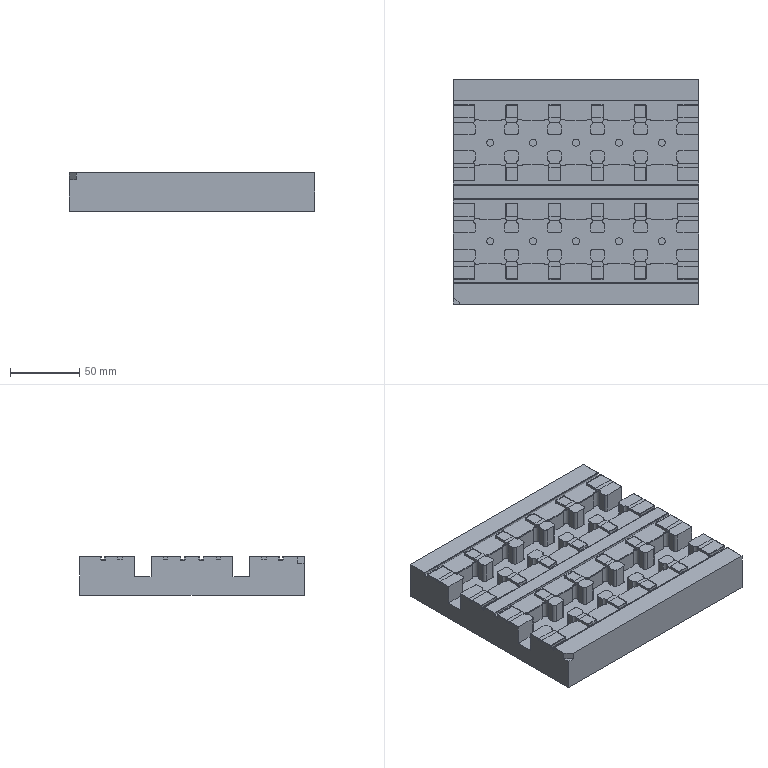NC program | NX | posted by the shop | part box 177 x 162 x 28 mm
Lines 249523 to 252035 of 254847:
N6 T04 M06
(D3  D=3. R=0. H=04 ce=0.05 di=0.02)
(D.N=04 MAX_Z=43. MIN_Z=25.32 Time=23.67M)
T17
G00 G90 G54 X94. Y64.15 M03 S5000
G43 H04 Z43.
M08
Z27.94
G01 X88.5 F1500.
X-88.5
X-94.
G00 Z27.88
G01 X-88.5
X88.5
X94.
G00 Z27.82
G01 X88.5
X-88.5
X-94.
G00 Z27.76
G01 X-88.5
X88.5
X94.
G00 Z27.7
G01 X88.5
X-88.5
X-94.
G00 Z27.64
G01 X-88.5
X88.5
X94.
G00 Z27.58
G01 X88.5
X-88.5
X-94.
G00 Z27.52
G01 X-88.5
X88.5
X94.
G00 Z27.46
G01 X88.5
X-88.5
X-94.
G00 Z27.4
G01 X-88.5
X88.5
X94.
G00 Z27.34
G01 X88.5
X-88.5
X-94.
G00 Z27.28
G01 X-88.5
X88.5
X94.
G00 Z27.22
G01 X88.5
X-88.5
X-94.
G00 Z27.16
G01 X-88.5
X88.5
X94.
G00 Z27.1
G01 X88.5
X-88.5
X-94.
G00 Z27.04
G01 X-88.5
X88.5
X94.
G00 Z26.98
G01 X88.5
X-88.5
X-94.
G00 Z26.92
G01 X-88.5
X88.5
X94.
G00 Z26.86
G01 X88.5
X-88.5
X-94.
G00 Z26.8
G01 X-88.5
X88.5
X94.
G00 Z26.74
G01 X88.5
X-88.5
X-94.
G00 Z26.68
G01 X-88.5
X88.5
X94.
G00 Z26.62
G01 X88.5
X-88.5
X-94.
G00 Z26.56
G01 X-88.5
X88.5
X94.
G00 Z26.5
G01 X88.5
X-88.5
X-94.
G00 Z26.44
G01 X-88.5
X88.5
X94.
G00 Z26.38
G01 X88.5
X-88.5
X-94.
G00 Z26.32
G01 X-88.5
X88.5
X94.
G00 Z26.26
G01 X88.5
X-88.5
X-94.
G00 Z26.2
G01 X-88.5
X88.5
X94.
G00 Z26.14
G01 X88.5
X-88.5
X-94.
G00 Z26.08
G01 X-88.5
X88.5
X94.
G00 Z26.02
G01 X88.5
X-88.5
X-94.
G00 Z25.96
G01 X-88.5
X88.5
X94.
G00 Z25.9
G01 X88.5
X-88.5
X-94.
G00 Z25.84
G01 X-88.5
X88.5
X94.
G00 Z25.78
G01 X88.5
X-88.5
X-94.
G00 Z25.72
G01 X-88.5
X88.5
X94.
G00 Z25.66
G01 X88.5
X-88.5
X-94.
G00 Z25.6
G01 X-88.5
X88.5
X94.
G00 Z25.54
G01 X88.5
X-88.5
X-94.
G00 Z25.48
G01 X-88.5
X88.5
X94.
G00 Z25.42
G01 X88.5
X-88.5
X-94.
G00 Z25.36
G01 X-88.5
X88.5
X94.
G00 Z25.32
G01 X88.5
X-88.5
X-94.
G00 Z43.
Y7.05
Z27.94
G01 X-88.5
X88.5
X94.
G00 Z27.88
G01 X88.5
X-88.5
X-94.
G00 Z27.82
G01 X-88.5
X88.5
X94.
G00 Z27.76
G01 X88.5
X-88.5
X-94.
G00 Z27.7
G01 X-88.5
X88.5
X94.
G00 Z27.64
G01 X88.5
X-88.5
X-94.
G00 Z27.58
G01 X-88.5
X88.5
X94.
G00 Z27.52
G01 X88.5
X-88.5
X-94.
G00 Z27.46
G01 X-88.5
X88.5
X94.
G00 Z27.4
G01 X88.5
X-88.5
X-94.
G00 Z27.34
G01 X-88.5
X88.5
X94.
G00 Z27.28
G01 X88.5
X-88.5
X-94.
G00 Z27.22
G01 X-88.5
X88.5
X94.
G00 Z27.16
G01 X88.5
X-88.5
X-94.
G00 Z27.1
G01 X-88.5
X88.5
X94.
G00 Z27.04
G01 X88.5
X-88.5
X-94.
G00 Z26.98
G01 X-88.5
X88.5
X94.
G00 Z26.92
G01 X88.5
X-88.5
X-94.
G00 Z26.86
G01 X-88.5
X88.5
X94.
G00 Z26.8
G01 X88.5
X-88.5
X-94.
G00 Z26.74
G01 X-88.5
X88.5
X94.
G00 Z26.68
G01 X88.5
X-88.5
X-94.
G00 Z26.62
G01 X-88.5
X88.5
X94.
G00 Z26.56
G01 X88.5
X-88.5
X-94.
G00 Z26.5
G01 X-88.5
X88.5
X94.
G00 Z26.44
G01 X88.5
X-88.5
X-94.
G00 Z26.38
G01 X-88.5
X88.5
X94.
G00 Z26.32
G01 X88.5
X-88.5
X-94.
G00 Z26.26
G01 X-88.5
X88.5
X94.
G00 Z26.2
G01 X88.5
X-88.5
X-94.
G00 Z26.14
G01 X-88.5
X88.5
X94.
G00 Z26.08
G01 X88.5
X-88.5
X-94.
G00 Z26.02
G01 X-88.5
X88.5
X94.
G00 Z25.96
G01 X88.5
X-88.5
X-94.
G00 Z25.9
G01 X-88.5
X88.5
X94.
G00 Z25.84
G01 X88.5
X-88.5
X-94.
G00 Z25.78
G01 X-88.5
X88.5
X94.
G00 Z25.72
G01 X88.5
X-88.5
X-94.
G00 Z25.66
G01 X-88.5
X88.5
X94.
G00 Z25.6
G01 X88.5
X-88.5
X-94.
G00 Z25.54
G01 X-88.5
X88.5
X94.
G00 Z25.48
G01 X88.5
X-88.5
X-94.
G00 Z25.42
G01 X-88.5
X88.5
X94.
G00 Z25.36
G01 X88.5
X-88.5
X-94.
G00 Z25.32
G01 X-88.5
X88.5
X94.
G00 Z43.
Y-7.05
Z27.94
G01 X88.5
X-88.5
X-94.
G00 Z27.88
G01 X-88.5
X88.5
X94.
G00 Z27.82
G01 X88.5
X-88.5
X-94.
G00 Z27.76
G01 X-88.5
X88.5
X94.
G00 Z27.7
G01 X88.5
X-88.5
X-94.
G00 Z27.64
G01 X-88.5
X88.5
X94.
G00 Z27.58
G01 X88.5
X-88.5
X-94.
G00 Z27.52
G01 X-88.5
X88.5
X94.
G00 Z27.46
G01 X88.5
X-88.5
X-94.
G00 Z27.4
G01 X-88.5
X88.5
X94.
G00 Z27.34
G01 X88.5
X-88.5
X-94.
G00 Z27.28
G01 X-88.5
X88.5
X94.
G00 Z27.22
G01 X88.5
X-88.5
X-94.
G00 Z27.16
G01 X-88.5
X88.5
X94.
G00 Z27.1
G01 X88.5
X-88.5
X-94.
G00 Z27.04
G01 X-88.5
X88.5
X94.
G00 Z26.98
G01 X88.5
X-88.5
X-94.
G00 Z26.92
G01 X-88.5
X88.5
X94.
G00 Z26.86
G01 X88.5
X-88.5
X-94.
G00 Z26.8
G01 X-88.5
X88.5
X94.
G00 Z26.74
G01 X88.5
X-88.5
X-94.
G00 Z26.68
G01 X-88.5
X88.5
X94.
G00 Z26.62
G01 X88.5
X-88.5
X-94.
G00 Z26.56
G01 X-88.5
X88.5
X94.
G00 Z26.5
G01 X88.5
X-88.5
X-94.
G00 Z26.44
G01 X-88.5
X88.5
X94.
G00 Z26.38
G01 X88.5
X-88.5
X-94.
G00 Z26.32
G01 X-88.5
X88.5
X94.
G00 Z26.26
G01 X88.5
X-88.5
X-94.
G00 Z26.2
G01 X-88.5
X88.5
X94.
G00 Z26.14
G01 X88.5
X-88.5
X-94.
G00 Z26.08
G01 X-88.5
X88.5
X94.
G00 Z26.02
G01 X88.5
X-88.5
X-94.
G00 Z25.96
G01 X-88.5
X88.5
X94.
G00 Z25.9
G01 X88.5
X-88.5
X-94.
G00 Z25.84
G01 X-88.5
X88.5
X94.
G00 Z25.78
G01 X88.5
X-88.5
X-94.
G00 Z25.72
G01 X-88.5
X88.5
X94.
G00 Z25.66
G01 X88.5
X-88.5
X-94.
G00 Z25.6
G01 X-88.5
X88.5
X94.
G00 Z25.54
G01 X88.5
X-88.5
X-94.
G00 Z25.48
G01 X-88.5
X88.5
X94.
G00 Z25.42
G01 X88.5
X-88.5
X-94.
G00 Z25.36
G01 X-88.5
X88.5
X94.
G00 Z25.32
G01 X88.5
X-88.5
X-94.
G00 Z43.
Y-64.15
Z27.94
G01 X-88.5
X88.5
X94.
G00 Z27.88
G01 X88.5
X-88.5
X-94.
G00 Z27.82
G01 X-88.5
X88.5
X94.
G00 Z27.76
G01 X88.5
X-88.5
X-94.
G00 Z27.7
G01 X-88.5
X88.5
X94.
G00 Z27.64
G01 X88.5
X-88.5
X-94.
G00 Z27.58
G01 X-88.5
X88.5
X94.
G00 Z27.52
G01 X88.5
X-88.5
X-94.
G00 Z27.46
G01 X-88.5
X88.5
X94.
G00 Z27.4
G01 X88.5
X-88.5
X-94.
G00 Z27.34
G01 X-88.5
X88.5
X94.
G00 Z27.28
G01 X88.5
X-88.5
X-94.
G00 Z27.22
G01 X-88.5
X88.5
X94.
G00 Z27.16
G01 X88.5
X-88.5
X-94.
G00 Z27.1
G01 X-88.5
X88.5
X94.
G00 Z27.04
G01 X88.5
X-88.5
X-94.
G00 Z26.98
G01 X-88.5
X88.5
X94.
G00 Z26.92
G01 X88.5
X-88.5
X-94.
G00 Z26.86
G01 X-88.5
X88.5
X94.
G00 Z26.8
G01 X88.5
X-88.5
X-94.
G00 Z26.74
G01 X-88.5
X88.5
X94.
G00 Z26.68
G01 X88.5
X-88.5
X-94.
G00 Z26.62
G01 X-88.5
X88.5
X94.
G00 Z26.56
G01 X88.5
X-88.5
X-94.
G00 Z26.5
G01 X-88.5
X88.5
X94.
G00 Z26.44
G01 X88.5
X-88.5
X-94.
G00 Z26.38
G01 X-88.5
X88.5
X94.
G00 Z26.32
G01 X88.5
X-88.5
X-94.
G00 Z26.26
G01 X-88.5
X88.5
X94.
G00 Z26.2
G01 X88.5
X-88.5
X-94.
G00 Z26.14
G01 X-88.5
X88.5
X94.
G00 Z26.08
G01 X88.5
X-88.5
X-94.
G00 Z26.02
G01 X-88.5
X88.5
X94.
G00 Z25.96
G01 X88.5
X-88.5
X-94.
G00 Z25.9
G01 X-88.5
X88.5
X94.
G00 Z25.84
G01 X88.5
X-88.5
X-94.
G00 Z25.78
G01 X-88.5
X88.5
X94.
G00 Z25.72
G01 X88.5
X-88.5
X-94.
G00 Z25.66
G01 X-88.5
X88.5
X94.
G00 Z25.6
G01 X88.5
X-88.5
X-94.
G00 Z25.54
G01 X-88.5
X88.5
X94.
G00 Z25.48
G01 X88.5
X-88.5
X-94.
G00 Z25.42
G01 X-88.5
X88.5
X94.
G00 Z25.36
G01 X88.5
X-88.5
X-94.
G00 Z25.32
G01 X-88.5
X88.5
X94.
G00 Z43.
G00 G90 X71.136 Y50.333 M03 S5000
Z40.
Z26.35
G01 Z25.35 F1000.
G41 D04
X71.276 Y50.475
G03 X71.45 Y50.897 I-.426 J.422
G01 Y64.15
X52.55
Y50.897
G03 X52.724 Y50.475 I.6 J0.0
G01 G40 X52.864 Y50.333
Z26.35
G00 Z40.
X40.136
Z26.35
G01 Z25.35
G41 D04
X40.276 Y50.475
G03 X40.45 Y50.897 I-.426 J.422
G01 Y64.15
X21.55
Y50.897
G03 X21.724 Y50.475 I.6 J0.0
G01 G40 X21.864 Y50.333
Z26.35
G00 Z40.
X9.136
Z26.35
G01 Z25.35
G41 D04
X9.276 Y50.475
G03 X9.45 Y50.897 I-.426 J.422
G01 Y64.15
X-9.45
Y50.897
G03 X-9.276 Y50.475 I.6 J0.0
G01 G40 X-9.136 Y50.333
Z26.35
G00 Z40.
X-21.864
Z26.35
G01 Z25.35
G41 D04
X-21.724 Y50.475
G03 X-21.55 Y50.897 I-.426 J.422
G01 Y64.15
X-40.45
Y50.897
G03 X-40.276 Y50.475 I.6 J0.0
G01 G40 X-40.136 Y50.333
Z26.35
G00 Z40.
X-52.864
Z26.35
G01 Z25.35
G41 D04
X-52.724 Y50.475
G03 X-52.55 Y50.897 I-.426 J.422
G01 Y64.15
X-71.45
Y50.897
G03 X-71.276 Y50.475 I.6 J0.0
G01 G40 X-71.136 Y50.333
Z26.35
G00 Z40.
X52.864 Y20.867
Z26.35
G01 Z25.35
G41 D04
X52.724 Y20.725
G03 X52.55 Y20.303 I.426 J-.422
G01 Y7.05
X71.45
Y20.303
G03 X71.276 Y20.725 I-.6 J0.0
G01 G40 X71.136 Y20.867
Z26.35
G00 Z40.
X21.864
Z26.35
G01 Z25.35
G41 D04
X21.724 Y20.725
G03 X21.55 Y20.303 I.426 J-.422
G01 Y7.05
X40.45
Y20.303
G03 X40.276 Y20.725 I-.6 J0.0
G01 G40 X40.136 Y20.867
Z26.35
G00 Z40.
X-9.136
Z26.35
G01 Z25.35
G41 D04
X-9.276 Y20.725
G03 X-9.45 Y20.303 I.426 J-.422
G01 Y7.05
X9.45
Y20.303
G03 X9.276 Y20.725 I-.6 J0.0
G01 G40 X9.136 Y20.867
Z26.35
G00 Z40.
X-40.136
Z26.35
G01 Z25.35
G41 D04
X-40.276 Y20.725
G03 X-40.45 Y20.303 I.426 J-.422
G01 Y7.05
X-21.55
Y20.303
G03 X-21.724 Y20.725 I-.6 J0.0
G01 G40 X-21.864 Y20.867
Z26.35
G00 Z40.
X-71.136
Z26.35
G01 Z25.35
G41 D04
X-71.276 Y20.725
G03 X-71.45 Y20.303 I.426 J-.422
G01 Y7.05
X-52.55
Y20.303
G03 X-52.724 Y20.725 I-.6 J0.0
G01 G40 X-52.864 Y20.867
Z26.35
G00 Z40.
Y-20.867
Z26.35
G01 Z25.35
G41 D04
X-52.724 Y-20.725
G03 X-52.55 Y-20.303 I-.426 J.422
G01 Y-7.05
X-71.45
Y-20.303
G03 X-71.276 Y-20.725 I.6 J0.0
G01 G40 X-71.136 Y-20.867
Z26.35
G00 Z40.
X-21.864
Z26.35
G01 Z25.35
G41 D04
X-21.724 Y-20.725
G03 X-21.55 Y-20.303 I-.426 J.422
G01 Y-7.05
X-40.45
Y-20.303
G03 X-40.276 Y-20.725 I.6 J0.0
G01 G40 X-40.136 Y-20.867
Z26.35
G00 Z40.
X9.136
Z26.35
G01 Z25.35
G41 D04
X9.276 Y-20.725
G03 X9.45 Y-20.303 I-.426 J.422
G01 Y-7.05
X-9.45
Y-20.303
G03 X-9.276 Y-20.725 I.6 J0.0
G01 G40 X-9.136 Y-20.867
Z26.35
G00 Z40.
X40.136
Z26.35
G01 Z25.35
G41 D04
X40.276 Y-20.725
G03 X40.45 Y-20.303 I-.426 J.422
G01 Y-7.05
X21.55
Y-20.303
G03 X21.724 Y-20.725 I.6 J0.0
G01 G40 X21.864 Y-20.867
Z26.35
G00 Z40.
X71.136
Z26.35
G01 Z25.35
G41 D04
X71.276 Y-20.725
G03 X71.45 Y-20.303 I-.426 J.422
G01 Y-7.05
X52.55
Y-20.303
G03 X52.724 Y-20.725 I.6 J0.0
G01 G40 X52.864 Y-20.867
Z26.35
G00 Z40.
Y-50.333
Z26.35
G01 Z25.35
G41 D04
X52.724 Y-50.475
G03 X52.55 Y-50.897 I.426 J-.422
G01 Y-64.15
X71.45
Y-50.897
G03 X71.276 Y-50.475 I-.6 J0.0
G01 G40 X71.136 Y-50.333
Z26.35
G00 Z40.
X21.864
Z26.35
G01 Z25.35
G41 D04
X21.724 Y-50.475
G03 X21.55 Y-50.897 I.426 J-.422
G01 Y-64.15
X40.45
Y-50.897
G03 X40.276 Y-50.475 I-.6 J0.0
G01 G40 X40.136 Y-50.333
Z26.35
G00 Z40.
X-9.136
Z26.35
G01 Z25.35
G41 D04
X-9.276 Y-50.475
G03 X-9.45 Y-50.897 I.426 J-.422
G01 Y-64.15
X9.45
Y-50.897
G03 X9.276 Y-50.475 I-.6 J0.0
G01 G40 X9.136 Y-50.333
Z26.35
G00 Z40.
X-40.136
Z26.35
G01 Z25.35
G41 D04
X-40.276 Y-50.475
G03 X-40.45 Y-50.897 I.426 J-.422
G01 Y-64.15
X-21.55
Y-50.897
G03 X-21.724 Y-50.475 I-.6 J0.0
G01 G40 X-21.864 Y-50.333
Z26.35
G00 Z40.
X-71.136
Z26.35
G01 Z25.35
G41 D04
X-71.276 Y-50.475
G03 X-71.45 Y-50.897 I.426 J-.422
G01 Y-64.15
X-52.55
Y-50.897
G03 X-52.724 Y-50.475 I-.6 J0.0
G01 G40 X-52.864 Y-50.333
Z26.35
G00 Z40.
G91 G28 Z0.0
M05
M09
G91 G28 Z0.0
M01
N7 T17 M06
(C6SpotDrill  D=6. R=0. H=17 ce=0.00 di=0.05)
(MAX_Z=43. MIN_Z=12.7 Time=0.33M)
T03
G00 G90 G54 X-62. Y-35.6 M03 S1500
G43 H17 Z43.
M08
G98 G81 X-62. Y-35.6 Z12.7 R14.5 F60.
X-31.
X0.0
X31.
X62.
Y35.6
X31.
X0.0
X-31.
X-62.
G80
G00 Z43.
G91 G28 Z0.0
M05
M09
G91 G28 Z0.0
M01
N8 T03 M06
(ZT5.1 D=5.1 DR_a=118 H=03)
(MAX_Z=43. MIN_Z=1.35 Time=1.12M)
T11
G00 G90 G54 X-62. Y-35.6 M03 S1200
G43 H03 Z43.
M08
G98 G83 X-62. Y-35.6 Z1.35 R14.5 F120. Q1.5
X-31.
X0.0
X31.
X62.
G98 G83 X62. Y35.6 Z1.6 R14.5 Q1.5
X31.
X0.0
X-31.
X-62.
G80
G00 Z43.
G91 G28 Z0.0
M05
M09
G91 G28 Z0.0
M01
N9 T11 M06
(D10-J  D=10. R=0. H=11 ce=0.00 di=0.00)
(MAX_Z=43. MIN_Z=28. Time=6.55M)
T14
G00 G90 G54 X98.5 Y-81.086 M03 S3000
G43 H11 Z43.
M08
Z30.
G01 Z28. F1000.
X93.5
X-93.5
Y-76.171
X93.5
Y-71.257
X-93.5
Y-66.343
X93.5
Y-61.429
X-93.5
Y-56.514
X93.5
Y-51.6
X-93.5
Y-46.686
X93.5
Y-41.771
X-93.5
Y-36.857
X93.5
Y-31.943
X-93.5
Y-27.029
X93.5
Y-22.114
X-93.5
Y-17.2
X93.5
Y-12.286
X-93.5
Y-7.371
X93.5
Y-2.457
X-93.5
Y2.457
X93.5
Y7.371
X-93.5
Y12.286
X93.5
Y17.2
X-93.5
Y22.114
X93.5
Y27.029
X-93.5
Y31.943
X93.5
Y36.857
X-93.5
Y41.771
X93.5
Y46.686
X-93.5
Y51.6
X93.5
Y56.514
X-93.5
Y61.429
X93.5
Y66.343
X-93.5
Y71.257
X93.5
Y76.171
X-93.5
Y81.086
X93.5
X98.5
Z30.
G00 Z43.
G91 G28 Z0.0
M05
M09
G91 G28 Z0.0
M01
N10 T14 M06
(D4-J  D=4. R=0. H=14 ce=0.30 di=0.00)
(MAX_Z=43. MIN_Z=13.5 Time=3.21M)
T13
G00 G90 G54 X-93.5 Y35.6 M03 S4000
G43 H14 Z43.
M08
Z14.
G01 Z13.5 F900.
X-88.9
Y39.3 F1000.
X-74.25
G03 X-69.95 Y43.6 I0.0 J4.3
G01 Y47.931
G03 X-70.334 Y49.204 I-2.3 J0.0
X-69.561 Y49.07 I.773 J2.166
G01 X-54.439
G03 X-53.666 Y49.204 I0.0 J2.3
X-54.05 Y47.931 I1.916 J-1.273
G01 Y43.6
G03 X-49.75 Y39.3 I4.3 J0.0
G01 X-43.25
G03 X-38.95 Y43.6 I0.0 J4.3
G01 Y47.931
G03 X-39.334 Y49.204 I-2.3 J0.0
X-38.561 Y49.07 I.773 J2.166
G01 X-23.439
G03 X-22.666 Y49.204 I0.0 J2.3
X-23.05 Y47.931 I1.916 J-1.273
G01 Y43.6
G03 X-18.75 Y39.3 I4.3 J0.0
G01 X-12.25
G03 X-7.95 Y43.6 I0.0 J4.3
G01 Y47.931
G03 X-8.334 Y49.204 I-2.3 J0.0
X-7.561 Y49.07 I.773 J2.166
G01 X7.561
G03 X8.334 Y49.204 I0.0 J2.3
X7.95 Y47.931 I1.916 J-1.273
G01 Y43.6
G03 X12.25 Y39.3 I4.3 J0.0
G01 X18.75
G03 X23.05 Y43.6 I0.0 J4.3
G01 Y47.931
G03 X22.666 Y49.204 I-2.3 J0.0
X23.439 Y49.07 I.773 J2.166
G01 X38.561
G03 X39.334 Y49.204 I0.0 J2.3
X38.95 Y47.931 I1.916 J-1.273
G01 Y43.6
G03 X43.25 Y39.3 I4.3 J0.0
G01 X49.75
G03 X54.05 Y43.6 I0.0 J4.3
G01 Y47.931
G03 X53.666 Y49.204 I-2.3 J0.0
X54.439 Y49.07 I.773 J2.166
G01 X69.561
G03 X70.334 Y49.204 I0.0 J2.3
X69.95 Y47.931 I1.916 J-1.273
G01 Y43.6
G03 X74.25 Y39.3 I4.3 J0.0
G01 X88.9
Y31.9
X74.25
G03 X69.95 Y27.6 I0.0 J-4.3
G01 Y23.269
G03 X70.334 Y21.996 I2.3 J0.0
X69.561 Y22.13 I-.773 J-2.166
G01 X54.439
G03 X53.666 Y21.996 I0.0 J-2.3
X54.05 Y23.269 I-1.916 J1.273
G01 Y27.6
G03 X49.75 Y31.9 I-4.3 J0.0
G01 X43.25
G03 X38.95 Y27.6 I0.0 J-4.3
G01 Y23.269
G03 X39.334 Y21.996 I2.3 J0.0
X38.561 Y22.13 I-.773 J-2.166
G01 X23.439
G03 X22.666 Y21.996 I0.0 J-2.3
X23.05 Y23.269 I-1.916 J1.273
G01 Y27.6
G03 X18.75 Y31.9 I-4.3 J0.0
G01 X12.25
G03 X7.95 Y27.6 I0.0 J-4.3
G01 Y23.269
G03 X8.334 Y21.996 I2.3 J0.0
X7.561 Y22.13 I-.773 J-2.166
G01 X-7.561
G03 X-8.334 Y21.996 I0.0 J-2.3
X-7.95 Y23.269 I-1.916 J1.273
G01 Y27.6
G03 X-12.25 Y31.9 I-4.3 J0.0
G01 X-18.75
G03 X-23.05 Y27.6 I0.0 J-4.3
G01 Y23.269
G03 X-22.666 Y21.996 I2.3 J0.0
X-23.439 Y22.13 I-.773 J-2.166
G01 X-38.561
G03 X-39.334 Y21.996 I0.0 J-2.3
X-38.95 Y23.269 I-1.916 J1.273
G01 Y27.6
G03 X-43.25 Y31.9 I-4.3 J0.0
G01 X-49.75
G03 X-54.05 Y27.6 I0.0 J-4.3
G01 Y23.269
G03 X-53.666 Y21.996 I2.3 J0.0
X-54.439 Y22.13 I-.773 J-2.166
G01 X-69.561
G03 X-70.334 Y21.996 I0.0 J-2.3
X-69.95 Y23.269 I-1.916 J1.273
G01 Y27.6
G03 X-74.25 Y31.9 I-4.3 J0.0
G01 X-88.9
Y35.6
X-86.8
Y37.2
X-74.25
G03 X-67.85 Y43.6 I0.0 J6.4
G01 Y46.97
X-56.15
Y43.6
G03 X-49.75 Y37.2 I6.4 J0.0
G01 X-43.25
G03 X-36.85 Y43.6 I0.0 J6.4
G01 Y46.97
X-25.15
Y43.6
G03 X-18.75 Y37.2 I6.4 J0.0
G01 X-12.25
G03 X-5.85 Y43.6 I0.0 J6.4
G01 Y46.97
X5.85
Y43.6
G03 X12.25 Y37.2 I6.4 J0.0
G01 X18.75
G03 X25.15 Y43.6 I0.0 J6.4
G01 Y46.97
X36.85
Y43.6
G03 X43.25 Y37.2 I6.4 J0.0
G01 X49.75
G03 X56.15 Y43.6 I0.0 J6.4
G01 Y46.97
X67.85
Y43.6
G03 X74.25 Y37.2 I6.4 J0.0
G01 X86.8
Y34.
X74.25
G03 X67.85 Y27.6 I0.0 J-6.4
G01 Y24.23
X56.15
Y27.6
G03 X52.91 Y33.165 I-6.4 J0.0
G01 X54.293 Y35.6
G03 X58.95 Y43.6 I-4.543 J8.
G01 Y44.17
X65.05
Y43.6
G03 X69.707 Y35.6 I9.2 J0.0
X65.05 Y27.6 I4.543 J-8.
G01 Y27.03
X58.95
Y27.6
G03 X54.293 Y35.6 I-9.2 J0.0
G01 X58.694
G03 X61.541 Y41.37 I-8.944 J8.
G01 X62.459
G03 X65.306 Y35.6 I11.791 J2.23
X62.459 Y29.83 I8.944 J-8.
G01 X61.541
G03 X58.694 Y35.6 I-11.791 J-2.23
G01 X60.995
G03 X62. Y37.246 I-11.245 J8.
X63.005 Y35.6 I12.25 J6.354
X62. Y33.954 I11.245 J-8.
X60.995 Y35.6 I-12.25 J-6.354
G01 X54.293
X52.91 Y33.165
G03 X49.75 Y34. I-3.16 J-5.565
G01 X43.25
G03 X36.85 Y27.6 I0.0 J-6.4
G01 Y24.23
X25.15
Y27.6
G03 X21.91 Y33.165 I-6.4 J0.0
G01 X23.293 Y35.6
G03 X27.95 Y43.6 I-4.543 J8.
G01 Y44.17
X34.05
Y43.6
G03 X38.707 Y35.6 I9.2 J0.0
X34.05 Y27.6 I4.543 J-8.
G01 Y27.03
X27.95
Y27.6
G03 X23.293 Y35.6 I-9.2 J0.0
G01 X27.694
G03 X30.541 Y41.37 I-8.944 J8.
G01 X31.459
G03 X34.306 Y35.6 I11.791 J2.23
X31.459 Y29.83 I8.944 J-8.
G01 X30.541
G03 X27.694 Y35.6 I-11.791 J-2.23
G01 X29.995
G03 X31. Y37.246 I-11.245 J8.
X32.005 Y35.6 I12.25 J6.354
X31. Y33.954 I11.245 J-8.
X29.995 Y35.6 I-12.25 J-6.354
G01 X23.293
X21.91 Y33.165
G03 X18.75 Y34. I-3.16 J-5.565
G01 X12.25
G03 X5.85 Y27.6 I0.0 J-6.4
G01 Y24.23
X-5.85
Y27.6
G03 X-9.09 Y33.165 I-6.4 J0.0
G01 X-7.707 Y35.6
G03 X-3.05 Y43.6 I-4.543 J8.
G01 Y44.17
X3.05
Y43.6
G03 X7.707 Y35.6 I9.2 J0.0
X3.05 Y27.6 I4.543 J-8.
G01 Y27.03
X-3.05
Y27.6
G03 X-7.707 Y35.6 I-9.2 J0.0
G01 X-3.306
G03 X-.459 Y41.37 I-8.944 J8.
G01 X.459
G03 X3.306 Y35.6 I11.791 J2.23
X.459 Y29.83 I8.944 J-8.
G01 X-.459
G03 X-3.306 Y35.6 I-11.791 J-2.23
G01 X-1.005
G03 X0.0 Y37.246 I-11.245 J8.
X1.005 Y35.6 I12.25 J6.354
X0.0 Y33.954 I11.245 J-8.
X-1.005 Y35.6 I-12.25 J-6.354
G01 X-7.707
X-9.09 Y33.165
G03 X-12.25 Y34. I-3.16 J-5.565
G01 X-18.75
G03 X-25.15 Y27.6 I0.0 J-6.4
G01 Y24.23
X-36.85
Y27.6
G03 X-40.09 Y33.165 I-6.4 J0.0
G01 X-38.707 Y35.6
G03 X-34.05 Y43.6 I-4.543 J8.
G01 Y44.17
X-27.95
Y43.6
G03 X-23.293 Y35.6 I9.2 J0.0
X-27.95 Y27.6 I4.543 J-8.
G01 Y27.03
X-34.05
Y27.6
G03 X-38.707 Y35.6 I-9.2 J0.0
G01 X-34.306
G03 X-31.459 Y41.37 I-8.944 J8.
G01 X-30.541
G03 X-27.694 Y35.6 I11.791 J2.23
X-30.541 Y29.83 I8.944 J-8.
G01 X-31.459
G03 X-34.306 Y35.6 I-11.791 J-2.23
G01 X-32.005
G03 X-31. Y37.246 I-11.245 J8.
X-29.995 Y35.6 I12.25 J6.354
X-31. Y33.954 I11.245 J-8.
X-32.005 Y35.6 I-12.25 J-6.354
G01 X-38.707
X-40.09 Y33.165
G03 X-43.25 Y34. I-3.16 J-5.565
G01 X-49.75
G03 X-56.15 Y27.6 I0.0 J-6.4
G01 Y24.23
X-67.85
Y27.6
G03 X-71.09 Y33.165 I-6.4 J0.0
G01 X-69.707 Y35.6
G03 X-65.05 Y43.6 I-4.543 J8.
G01 Y44.17
X-58.95
Y43.6
G03 X-54.293 Y35.6 I9.2 J0.0
X-58.95 Y27.6 I4.543 J-8.
G01 Y27.03
X-65.05
Y27.6
G03 X-69.707 Y35.6 I-9.2 J0.0
G01 X-65.306
G03 X-62.459 Y41.37 I-8.944 J8.
G01 X-61.541
G03 X-58.694 Y35.6 I11.791 J2.23
X-61.541 Y29.83 I8.944 J-8.
G01 X-62.459
G03 X-65.306 Y35.6 I-11.791 J-2.23
G01 X-63.005
G03 X-62. Y37.246 I-11.245 J8.
X-60.995 Y35.6 I12.25 J6.354
X-62. Y33.954 I11.245 J-8.
X-63.005 Y35.6 I-12.25 J-6.354
G01 X-69.707
X-71.09 Y33.165
G03 X-74.25 Y34. I-3.16 J-5.565
G01 X-86.8
Y35.6
Y36.1
X-93.5
Z14.
G00 Z43.
Y-35.6
Z14.
G01 Z13.5 F900.
X-88.9
Y-31.9 F1000.
X-74.25
G03 X-69.95 Y-27.6 I0.0 J4.3
G01 Y-23.269
G03 X-70.334 Y-21.996 I-2.3 J0.0
X-69.561 Y-22.13 I.773 J2.166
G01 X-54.439
G03 X-53.666 Y-21.996 I0.0 J2.3
X-54.05 Y-23.269 I1.916 J-1.273
G01 Y-27.6
G03 X-49.75 Y-31.9 I4.3 J0.0
G01 X-43.25
G03 X-38.95 Y-27.6 I0.0 J4.3
G01 Y-23.269
G03 X-39.334 Y-21.996 I-2.3 J0.0
X-38.561 Y-22.13 I.773 J2.166
G01 X-23.439
G03 X-22.666 Y-21.996 I0.0 J2.3
X-23.05 Y-23.269 I1.916 J-1.273
G01 Y-27.6
G03 X-18.75 Y-31.9 I4.3 J0.0
G01 X-12.25
G03 X-7.95 Y-27.6 I0.0 J4.3
G01 Y-23.269
G03 X-8.334 Y-21.996 I-2.3 J0.0
X-7.561 Y-22.13 I.773 J2.166
G01 X7.561
G03 X8.334 Y-21.996 I0.0 J2.3
X7.95 Y-23.269 I1.916 J-1.273
G01 Y-27.6
G03 X12.25 Y-31.9 I4.3 J0.0
G01 X18.75
G03 X23.05 Y-27.6 I0.0 J4.3
G01 Y-23.269
G03 X22.666 Y-21.996 I-2.3 J0.0
X23.439 Y-22.13 I.773 J2.166
G01 X38.561
G03 X39.334 Y-21.996 I0.0 J2.3
X38.95 Y-23.269 I1.916 J-1.273
G01 Y-27.6
G03 X43.25 Y-31.9 I4.3 J0.0
G01 X49.75
G03 X54.05 Y-27.6 I0.0 J4.3
G01 Y-23.269
G03 X53.666 Y-21.996 I-2.3 J0.0
X54.439 Y-22.13 I.773 J2.166
G01 X69.561
G03 X70.334 Y-21.996 I0.0 J2.3
X69.95 Y-23.269 I1.916 J-1.273
G01 Y-27.6
G03 X74.25 Y-31.9 I4.3 J0.0
G01 X88.9
Y-39.3
X74.25
G03 X69.95 Y-43.6 I0.0 J-4.3
G01 Y-47.931
G03 X70.334 Y-49.204 I2.3 J0.0
X69.561 Y-49.07 I-.773 J-2.166
G01 X54.439
G03 X53.666 Y-49.204 I0.0 J-2.3
X54.05 Y-47.931 I-1.916 J1.273
G01 Y-43.6
G03 X49.75 Y-39.3 I-4.3 J0.0
G01 X43.25
G03 X38.95 Y-43.6 I0.0 J-4.3
G01 Y-47.931
G03 X39.334 Y-49.204 I2.3 J0.0
X38.561 Y-49.07 I-.773 J-2.166
G01 X23.439
G03 X22.666 Y-49.204 I0.0 J-2.3
X23.05 Y-47.931 I-1.916 J1.273
G01 Y-43.6
G03 X18.75 Y-39.3 I-4.3 J0.0
G01 X12.25
G03 X7.95 Y-43.6 I0.0 J-4.3
G01 Y-47.931
G03 X8.334 Y-49.204 I2.3 J0.0
X7.561 Y-49.07 I-.773 J-2.166
G01 X-7.561
G03 X-8.334 Y-49.204 I0.0 J-2.3
X-7.95 Y-47.931 I-1.916 J1.273
G01 Y-43.6
G03 X-12.25 Y-39.3 I-4.3 J0.0
G01 X-18.75
G03 X-23.05 Y-43.6 I0.0 J-4.3
G01 Y-47.931
G03 X-22.666 Y-49.204 I2.3 J0.0
X-23.439 Y-49.07 I-.773 J-2.166
G01 X-38.561
G03 X-39.334 Y-49.204 I0.0 J-2.3
X-38.95 Y-47.931 I-1.916 J1.273
G01 Y-43.6
G03 X-43.25 Y-39.3 I-4.3 J0.0
G01 X-49.75
G03 X-54.05 Y-43.6 I0.0 J-4.3
G01 Y-47.931
G03 X-53.666 Y-49.204 I2.3 J0.0
X-54.439 Y-49.07 I-.773 J-2.166
G01 X-69.561
G03 X-70.334 Y-49.204 I0.0 J-2.3
X-69.95 Y-47.931 I-1.916 J1.273
G01 Y-43.6
G03 X-74.25 Y-39.3 I-4.3 J0.0
G01 X-88.9
Y-35.6
X-86.8
Y-34.
X-74.25
G03 X-67.85 Y-27.6 I0.0 J6.4
G01 Y-24.23
X-56.15
Y-27.6
G03 X-49.75 Y-34. I6.4 J0.0
G01 X-43.25
G03 X-36.85 Y-27.6 I0.0 J6.4
G01 Y-24.23
X-25.15
Y-27.6
G03 X-18.75 Y-34. I6.4 J0.0
G01 X-12.25
G03 X-5.85 Y-27.6 I0.0 J6.4
G01 Y-24.23
X5.85
Y-27.6
G03 X12.25 Y-34. I6.4 J0.0
G01 X18.75
G03 X25.15 Y-27.6 I0.0 J6.4
G01 Y-24.23
X36.85
Y-27.6
G03 X43.25 Y-34. I6.4 J0.0
G01 X49.75
G03 X56.15 Y-27.6 I0.0 J6.4
G01 Y-24.23
X67.85
Y-27.6
G03 X74.25 Y-34. I6.4 J0.0
G01 X86.8
Y-37.2
X74.25
G03 X67.85 Y-43.6 I0.0 J-6.4
G01 Y-46.97
X56.15
Y-43.6
G03 X52.91 Y-38.035 I-6.4 J0.0
G01 X54.293 Y-35.6
G03 X58.95 Y-27.6 I-4.543 J8.
G01 Y-27.03
X65.05
Y-27.6
G03 X69.707 Y-35.6 I9.2 J0.0
X65.05 Y-43.6 I4.543 J-8.
G01 Y-44.17
X58.95
Y-43.6
G03 X54.293 Y-35.6 I-9.2 J0.0
G01 X58.694
G03 X61.541 Y-29.83 I-8.944 J8.
G01 X62.459
G03 X65.306 Y-35.6 I11.791 J2.23
X62.459 Y-41.37 I8.944 J-8.
G01 X61.541
G03 X58.694 Y-35.6 I-11.791 J-2.23
G01 X60.995
G03 X62. Y-33.954 I-11.245 J8.
X63.005 Y-35.6 I12.25 J6.354
X62. Y-37.246 I11.245 J-8.
X60.995 Y-35.6 I-12.25 J-6.354
G01 X54.293
X52.91 Y-38.035
G03 X49.75 Y-37.2 I-3.16 J-5.565
G01 X43.25
G03 X36.85 Y-43.6 I0.0 J-6.4
G01 Y-46.97
X25.15
Y-43.6
G03 X21.91 Y-38.035 I-6.4 J0.0
G01 X23.293 Y-35.6
G03 X27.95 Y-27.6 I-4.543 J8.
G01 Y-27.03
X34.05
Y-27.6
G03 X38.707 Y-35.6 I9.2 J0.0
X34.05 Y-43.6 I4.543 J-8.
G01 Y-44.17
X27.95
Y-43.6
G03 X23.293 Y-35.6 I-9.2 J0.0
G01 X27.694
G03 X30.541 Y-29.83 I-8.944 J8.
G01 X31.459
G03 X34.306 Y-35.6 I11.791 J2.23
X31.459 Y-41.37 I8.944 J-8.
G01 X30.541
G03 X27.694 Y-35.6 I-11.791 J-2.23
G01 X29.995
G03 X31. Y-33.954 I-11.245 J8.
X32.005 Y-35.6 I12.25 J6.354
X31. Y-37.246 I11.245 J-8.
X29.995 Y-35.6 I-12.25 J-6.354
G01 X23.293
X21.91 Y-38.035
G03 X18.75 Y-37.2 I-3.16 J-5.565
G01 X12.25
G03 X5.85 Y-43.6 I0.0 J-6.4
G01 Y-46.97
X-5.85
Y-43.6
G03 X-9.09 Y-38.035 I-6.4 J0.0
G01 X-7.707 Y-35.6
G03 X-3.05 Y-27.6 I-4.543 J8.
G01 Y-27.03
X3.05
Y-27.6
G03 X7.707 Y-35.6 I9.2 J0.0
X3.05 Y-43.6 I4.543 J-8.
G01 Y-44.17
X-3.05
Y-43.6
G03 X-7.707 Y-35.6 I-9.2 J0.0
G01 X-3.306
G03 X-.459 Y-29.83 I-8.944 J8.
G01 X.459
G03 X3.306 Y-35.6 I11.791 J2.23
X.459 Y-41.37 I8.944 J-8.
G01 X-.459
G03 X-3.306 Y-35.6 I-11.791 J-2.23
G01 X-1.005
G03 X0.0 Y-33.954 I-11.245 J8.
X1.005 Y-35.6 I12.25 J6.354
X0.0 Y-37.246 I11.245 J-8.
X-1.005 Y-35.6 I-12.25 J-6.354
G01 X-7.707
X-9.09 Y-38.035
G03 X-12.25 Y-37.2 I-3.16 J-5.565
G01 X-18.75
G03 X-25.15 Y-43.6 I0.0 J-6.4
G01 Y-46.97
X-36.85
Y-43.6
G03 X-40.09 Y-38.035 I-6.4 J0.0
G01 X-38.707 Y-35.6
G03 X-34.05 Y-27.6 I-4.543 J8.
G01 Y-27.03
X-27.95
Y-27.6
G03 X-23.293 Y-35.6 I9.2 J0.0
X-27.95 Y-43.6 I4.543 J-8.
G01 Y-44.17
X-34.05
Y-43.6
G03 X-38.707 Y-35.6 I-9.2 J0.0
G01 X-34.306
G03 X-31.459 Y-29.83 I-8.944 J8.
G01 X-30.541
G03 X-27.694 Y-35.6 I11.791 J2.23
X-30.541 Y-41.37 I8.944 J-8.
G01 X-31.459
G03 X-34.306 Y-35.6 I-11.791 J-2.23
G01 X-32.005
G03 X-31. Y-33.954 I-11.245 J8.
X-29.995 Y-35.6 I12.25 J6.354
X-31. Y-37.246 I11.245 J-8.
X-32.005 Y-35.6 I-12.25 J-6.354
G01 X-38.707
X-40.09 Y-38.035
G03 X-43.25 Y-37.2 I-3.16 J-5.565
G01 X-49.75
G03 X-56.15 Y-43.6 I0.0 J-6.4
G01 Y-46.97
X-67.85
Y-43.6
G03 X-71.09 Y-38.035 I-6.4 J0.0
G01 X-69.707 Y-35.6
G03 X-65.05 Y-27.6 I-4.543 J8.
G01 Y-27.03
X-58.95
Y-27.6
G03 X-54.293 Y-35.6 I9.2 J0.0
X-58.95 Y-43.6 I4.543 J-8.
G01 Y-44.17
X-65.05
Y-43.6
G03 X-69.707 Y-35.6 I-9.2 J0.0
G01 X-65.306
G03 X-62.459 Y-29.83 I-8.944 J8.
G01 X-61.541
G03 X-58.694 Y-35.6 I11.791 J2.23
X-61.541 Y-41.37 I8.944 J-8.
G01 X-62.459
G03 X-65.306 Y-35.6 I-11.791 J-2.23
G01 X-63.005
G03 X-62. Y-33.954 I-11.245 J8.
X-60.995 Y-35.6 I12.25 J6.354
X-62. Y-37.246 I11.245 J-8.
X-63.005 Y-35.6 I-12.25 J-6.354
G01 X-69.707
X-71.09 Y-38.035
G03 X-74.25 Y-37.2 I-3.16 J-5.565
G01 X-86.8
Y-35.6
Y-35.1
X-93.5
Z14.
G00 Z43.
G91 G28 Z0.0
M05
M09
G91 G28 Z0.0
M01
N11 T13 M06
(D3-J  D=3. R=0. H=13 ce=0.30 di=0.00)
(MAX_Z=43. MIN_Z=25.3 Time=3.51M)
T01
G00 G90 G54 X62. Y-46.87 M03 S4000
G43 H13 Z43.
M08
Z25.8
G01 Z25.3 F900.
Y-51.07
X69.722 F1000.
X69.811 Y-51.204
G03 X71.2 Y-52.078 I1.666 J1.107
G01 Y-63.9
X52.8
Y-52.078
G03 X54.189 Y-51.204 I-.277 J1.981
G01 X54.278 Y-51.07
X62.
Y-53.17
X68.763
G03 X69.1 Y-53.438 I2.714 J3.073
G01 Y-61.8
X54.9
Y-53.438
G03 X55.237 Y-53.17 I-2.377 J3.34
G01 X62.
Y-55.27
X67.
Y-59.7
X57.
Y-55.27
X62.
Y-57.37
X64.9
Y-57.6
X59.1
Y-57.37
X62.
X62.5
Y-46.87
Z25.8
G00 Z43.
X31.
Z25.8
G01 Z25.3 F900.
Y-51.07
X38.722 F1000.
X38.811 Y-51.204
G03 X40.2 Y-52.078 I1.666 J1.107
G01 Y-63.9
X21.8
Y-52.078
G03 X23.189 Y-51.204 I-.277 J1.981
G01 X23.278 Y-51.07
X31.
Y-53.17
X37.763
G03 X38.1 Y-53.438 I2.714 J3.073
G01 Y-61.8
X23.9
Y-53.438
G03 X24.237 Y-53.17 I-2.377 J3.34
G01 X31.
Y-55.27
X36.
Y-59.7
X26.
Y-55.27
X31.
Y-57.37
X33.9
Y-57.6
X28.1
Y-57.37
X31.
X31.5
Y-46.87
Z25.8
G00 Z43.
X0.0
Z25.8
G01 Z25.3 F900.
Y-51.07
X7.722 F1000.
X7.811 Y-51.204
G03 X9.2 Y-52.078 I1.666 J1.107
G01 Y-63.9
X-9.2
Y-52.078
G03 X-7.811 Y-51.204 I-.277 J1.981
G01 X-7.722 Y-51.07
X0.0
Y-53.17
X6.763
G03 X7.1 Y-53.438 I2.714 J3.073
G01 Y-61.8
X-7.1
Y-53.438
G03 X-6.763 Y-53.17 I-2.377 J3.34
G01 X0.0
Y-55.27
X5.
Y-59.7
X-5.
Y-55.27
X0.0
Y-57.37
X2.9
Y-57.6
X-2.9
Y-57.37
X0.0
X.5
Y-46.87
Z25.8
G00 Z43.
X-31.
Z25.8
G01 Z25.3 F900.
Y-51.07
X-23.278 F1000.
X-23.189 Y-51.204
G03 X-21.8 Y-52.078 I1.666 J1.107
G01 Y-63.9
X-40.2
Y-52.078
G03 X-38.811 Y-51.204 I-.277 J1.981
G01 X-38.722 Y-51.07
X-31.
Y-53.17
X-24.237
G03 X-23.9 Y-53.438 I2.714 J3.073
G01 Y-61.8
X-38.1
Y-53.438
G03 X-37.763 Y-53.17 I-2.377 J3.34
G01 X-31.
Y-55.27
X-26.
Y-59.7
X-36.
Y-55.27
X-31.
Y-57.37
X-28.1
Y-57.6
X-33.9
Y-57.37
X-31.
X-30.5
Y-46.87
Z25.8
G00 Z43.
X-62.
Z25.8
G01 Z25.3 F900.
Y-51.07
X-54.278 F1000.
X-54.189 Y-51.204
G03 X-52.8 Y-52.078 I1.666 J1.107
G01 Y-63.9
X-71.2
Y-52.078
G03 X-69.811 Y-51.204 I-.277 J1.981
G01 X-69.722 Y-51.07
X-62.
Y-53.17
X-55.237
G03 X-54.9 Y-53.438 I2.714 J3.073
G01 Y-61.8
X-69.1
Y-53.438
G03 X-68.763 Y-53.17 I-2.377 J3.34
G01 X-62.
Y-55.27
X-57.
Y-59.7
X-67.
Y-55.27
X-62.
Y-57.37
X-59.1
Y-57.6
X-64.9
Y-57.37
X-62.
X-61.5
Y-46.87
Z25.8
G00 Z43.
X-62. Y-24.33
Z25.8
G01 Z25.3 F900.
Y-20.13
X-69.722 F1000.
X-69.811 Y-19.996
G03 X-71.2 Y-19.122 I-1.666 J-1.107
G01 Y-7.3
X-52.8
Y-19.122
G03 X-54.189 Y-19.996 I.277 J-1.981
G01 X-54.278 Y-20.13
X-62.
Y-18.03
X-68.763
G03 X-69.1 Y-17.762 I-2.714 J-3.073
G01 Y-9.4
X-54.9
Y-17.762
G03 X-55.237 Y-18.03 I2.377 J-3.34
G01 X-62.
Y-15.93
X-67.
Y-11.5
X-57.
Y-15.93
X-62.
Y-13.83
X-64.9
Y-13.6
X-59.1
Y-13.83
X-62.
X-62.5
Y-24.33
Z25.8
G00 Z43.
X-31.
Z25.8
G01 Z25.3 F900.
Y-20.13
X-38.722 F1000.
X-38.811 Y-19.996
G03 X-40.2 Y-19.122 I-1.666 J-1.107
G01 Y-7.3
X-21.8
Y-19.122
G03 X-23.189 Y-19.996 I.277 J-1.981
G01 X-23.278 Y-20.13
X-31.
Y-18.03
X-37.763
G03 X-38.1 Y-17.762 I-2.714 J-3.073
G01 Y-9.4
X-23.9
Y-17.762
G03 X-24.237 Y-18.03 I2.377 J-3.34
G01 X-31.
Y-15.93
X-36.
Y-11.5
X-26.
Y-15.93
X-31.
Y-13.83
X-33.9
Y-13.6
X-28.1
Y-13.83
X-31.
X-31.5
Y-24.33
Z25.8
G00 Z43.
X0.0
Z25.8
G01 Z25.3 F900.
Y-20.13
X-7.722 F1000.
X-7.811 Y-19.996
G03 X-9.2 Y-19.122 I-1.666 J-1.107
G01 Y-7.3
X9.2
Y-19.122
G03 X7.811 Y-19.996 I.277 J-1.981
G01 X7.722 Y-20.13
X0.0
Y-18.03
X-6.763
G03 X-7.1 Y-17.762 I-2.714 J-3.073
G01 Y-9.4
X7.1
Y-17.762
G03 X6.763 Y-18.03 I2.377 J-3.34
G01 X0.0
Y-15.93
X-5.
Y-11.5
X5.
Y-15.93
X0.0
Y-13.83
X-2.9
Y-13.6
X2.9
Y-13.83
X0.0
X-.5
Y-24.33
Z25.8
G00 Z43.
X31.
Z25.8
G01 Z25.3 F900.
Y-20.13
X23.278 F1000.
X23.189 Y-19.996
G03 X21.8 Y-19.122 I-1.666 J-1.107
G01 Y-7.3
X40.2
Y-19.122
G03 X38.811 Y-19.996 I.277 J-1.981
G01 X38.722 Y-20.13
X31.
Y-18.03
X24.237
G03 X23.9 Y-17.762 I-2.714 J-3.073
G01 Y-9.4
X38.1
Y-17.762
G03 X37.763 Y-18.03 I2.377 J-3.34
G01 X31.
Y-15.93
X26.
Y-11.5
X36.
Y-15.93
X31.
Y-13.83
X28.1
Y-13.6
X33.9
Y-13.83
X31.
X30.5
Y-24.33
Z25.8
G00 Z43.
X62.
Z25.8
G01 Z25.3 F900.
Y-20.13
X54.278 F1000.
X54.189 Y-19.996
G03 X52.8 Y-19.122 I-1.666 J-1.107
G01 Y-7.3
X71.2
Y-19.122
G03 X69.811 Y-19.996 I.277 J-1.981
G01 X69.722 Y-20.13
X62.
Y-18.03
X55.237
G03 X54.9 Y-17.762 I-2.714 J-3.073
G01 Y-9.4
X69.1
Y-17.762
G03 X68.763 Y-18.03 I2.377 J-3.34
G01 X62.
Y-15.93
X57.
Y-11.5
X67.
Y-15.93
X62.
Y-13.83
X59.1
Y-13.6
X64.9
Y-13.83
X62.
X61.5
Y-24.33
Z25.8
G00 Z43.
X62. Y24.33
Z25.8
G01 Z25.3 F900.
Y20.13
X69.722 F1000.
X69.811 Y19.996
G03 X71.2 Y19.122 I1.666 J1.107
G01 Y7.3
X52.8
Y19.122
G03 X54.189 Y19.996 I-.277 J1.981
G01 X54.278 Y20.13
X62.
Y18.03
X68.763
G03 X69.1 Y17.762 I2.714 J3.073
G01 Y9.4
X54.9
Y17.762
G03 X55.237 Y18.03 I-2.377 J3.34
G01 X62.
Y15.93
X67.
Y11.5
X57.
Y15.93
X62.
Y13.83
X64.9
Y13.6
X59.1
Y13.83
X62.
X62.5
Y24.33
Z25.8
G00 Z43.
X31.
Z25.8
G01 Z25.3 F900.
Y20.13
X38.722 F1000.
X38.811 Y19.996
G03 X40.2 Y19.122 I1.666 J1.107
G01 Y7.3
X21.8
Y19.122
G03 X23.189 Y19.996 I-.277 J1.981
G01 X23.278 Y20.13
X31.
Y18.03
X37.763
G03 X38.1 Y17.762 I2.714 J3.073
G01 Y9.4
X23.9
Y17.762
G03 X24.237 Y18.03 I-2.377 J3.34
G01 X31.
Y15.93
X36.
Y11.5
X26.
Y15.93
X31.
Y13.83
X33.9
Y13.6
X28.1
Y13.83
X31.
X31.5
Y24.33
Z25.8
G00 Z43.
X0.0
Z25.8
G01 Z25.3 F900.
Y20.13
X7.722 F1000.
X7.811 Y19.996
G03 X9.2 Y19.122 I1.666 J1.107
G01 Y7.3
X-9.2
Y19.122
G03 X-7.811 Y19.996 I-.277 J1.981
G01 X-7.722 Y20.13
X0.0
Y18.03
X6.763
G03 X7.1 Y17.762 I2.714 J3.073
G01 Y9.4
X-7.1
Y17.762
G03 X-6.763 Y18.03 I-2.377 J3.34
G01 X0.0
Y15.93
X5.
Y11.5
X-5.
Y15.93
X0.0
Y13.83
X2.9
Y13.6
X-2.9
Y13.83
X0.0
X.5
Y24.33
Z25.8
G00 Z43.
X-31.
Z25.8
G01 Z25.3 F900.
Y20.13
X-23.278 F1000.
X-23.189 Y19.996
G03 X-21.8 Y19.122 I1.666 J1.107
G01 Y7.3
X-40.2
Y19.122
G03 X-38.811 Y19.996 I-.277 J1.981
G01 X-38.722 Y20.13
X-31.
Y18.03
X-24.237
G03 X-23.9 Y17.762 I2.714 J3.073
G01 Y9.4
X-38.1
Y17.762
G03 X-37.763 Y18.03 I-2.377 J3.34
G01 X-31.
Y15.93
X-26.
Y11.5
X-36.
Y15.93
X-31.
Y13.83
X-28.1
Y13.6
X-33.9
Y13.83
X-31.
X-30.5
Y24.33
Z25.8
G00 Z43.
X-62.
Z25.8
G01 Z25.3 F900.
Y20.13
X-54.278 F1000.
X-54.189 Y19.996
G03 X-52.8 Y19.122 I1.666 J1.107
G01 Y7.3
X-71.2
Y19.122
G03 X-69.811 Y19.996 I-.277 J1.981
G01 X-69.722 Y20.13
X-62.
Y18.03
X-55.237
G03 X-54.9 Y17.762 I2.714 J3.073
G01 Y9.4
X-69.1
Y17.762
G03 X-68.763 Y18.03 I-2.377 J3.34
G01 X-62.
Y15.93
X-57.
Y11.5
X-67.
Y15.93
X-62.
Y13.83
X-59.1
Y13.6
X-64.9
Y13.83
X-62.
X-61.5
Y24.33
Z25.8
G00 Z43.
X62. Y46.87
Z25.8
G01 Z25.3 F900.
Y51.07
X54.278 F1000.
X54.189 Y51.204
G03 X52.8 Y52.078 I-1.666 J-1.107
G01 Y63.9
X71.2
Y52.078
G03 X69.811 Y51.204 I.277 J-1.981
G01 X69.722 Y51.07
X62.
Y53.17
X55.237
G03 X54.9 Y53.438 I-2.714 J-3.073
G01 Y61.8
X69.1
Y53.438
G03 X68.763 Y53.17 I2.377 J-3.34
G01 X62.
Y55.27
X57.
Y59.7
X67.
Y55.27
X62.
Y57.37
X59.1
Y57.6
X64.9
Y57.37
X62.
X61.5
Y46.87
Z25.8
G00 Z43.
X31.
Z25.8
G01 Z25.3 F900.
Y51.07
X23.278 F1000.
X23.189 Y51.204
G03 X21.8 Y52.078 I-1.666 J-1.107
G01 Y63.9
X40.2
Y52.078
G03 X38.811 Y51.204 I.277 J-1.981
G01 X38.722 Y51.07
X31.
Y53.17
X24.237
G03 X23.9 Y53.438 I-2.714 J-3.073
G01 Y61.8
X38.1
Y53.438
G03 X37.763 Y53.17 I2.377 J-3.34
G01 X31.
Y55.27
X26.
Y59.7
X36.
Y55.27
X31.
Y57.37
X28.1
Y57.6
X33.9
Y57.37
X31.
X30.5
Y46.87
Z25.8
G00 Z43.
X0.0
Z25.8
G01 Z25.3 F900.
Y51.07
X-7.722 F1000.
X-7.811 Y51.204
G03 X-9.2 Y52.078 I-1.666 J-1.107
G01 Y63.9
X9.2
Y52.078
G03 X7.811 Y51.204 I.277 J-1.981
G01 X7.722 Y51.07
X0.0
Y53.17
X-6.763
G03 X-7.1 Y53.438 I-2.714 J-3.073
G01 Y61.8
X7.1
Y53.438
G03 X6.763 Y53.17 I2.377 J-3.34
G01 X0.0
Y55.27
X-5.
Y59.7
X5.
Y55.27
X0.0
Y57.37
X-2.9
Y57.6
X2.9
Y57.37
X0.0
X-.5
Y46.87
Z25.8
G00 Z43.
X-31.
Z25.8
G01 Z25.3 F900.
Y51.07
X-38.722 F1000.
X-38.811 Y51.204
G03 X-40.2 Y52.078 I-1.666 J-1.107
G01 Y63.9
X-21.8
Y52.078
G03 X-23.189 Y51.204 I.277 J-1.981
G01 X-23.278 Y51.07
X-31.
Y53.17
X-37.763
G03 X-38.1 Y53.438 I-2.714 J-3.073
G01 Y61.8
X-23.9
Y53.438
G03 X-24.237 Y53.17 I2.377 J-3.34
G01 X-31.
Y55.27
X-36.
Y59.7
X-26.
Y55.27
X-31.
Y57.37
X-33.9
Y57.6
X-28.1
Y57.37
X-31.
X-31.5
Y46.87
Z25.8
G00 Z43.
X-62.
Z25.8
G01 Z25.3 F900.
Y51.07
X-69.722 F1000.
X-69.811 Y51.204
G03 X-71.2 Y52.078 I-1.666 J-1.107
G01 Y63.9
X-52.8
Y52.078
G03 X-54.189 Y51.204 I.277 J-1.981
G01 X-54.278 Y51.07
X-62.
Y53.17
X-68.763
G03 X-69.1 Y53.438 I-2.714 J-3.073
G01 Y61.8
X-54.9
Y53.438
G03 X-55.237 Y53.17 I2.377 J-3.34
G01 X-62.
Y55.27
X-67.
Y59.7
X-57.
Y55.27
X-62.
Y57.37
X-64.9
Y57.6
X-59.1
Y57.37
X-62.
X-62.5
Y46.87
Z25.8
G00 Z43.
G91 G28 Z0.0
M05
M09
G91 G28 Z0.0
M01